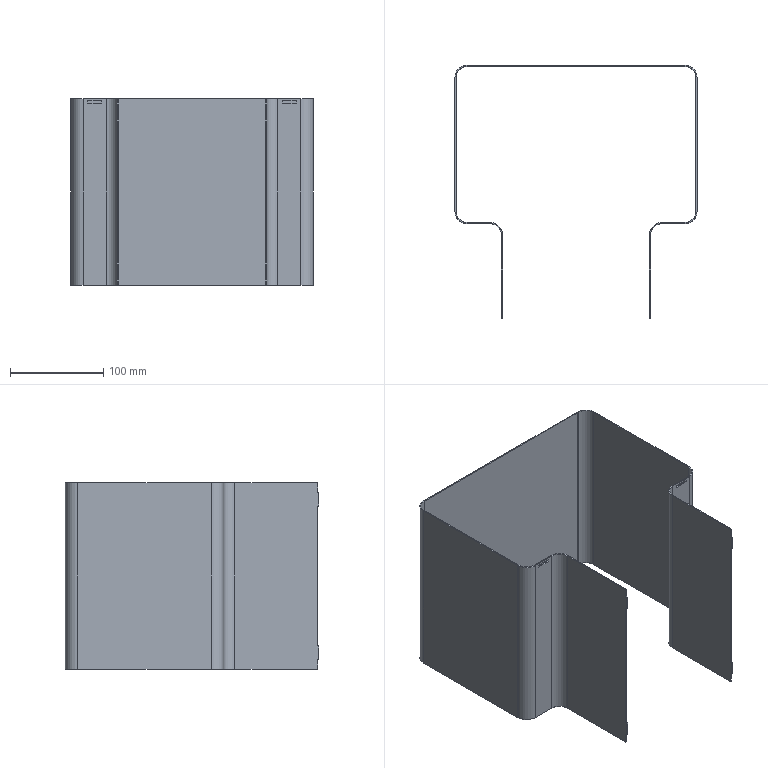Part | SolidWorks | features ICE 2, SMBaseFlange 2, FlatPattern 1, MirrorPattern 1, SheetMetal 1 | 1 solid | 78 faces | box 260 x 272 x 200 mm | volume 208024 mm3 | plane 66 | cylinder 12 | commonest cylinder face diameters 24 x6 26.4 x6